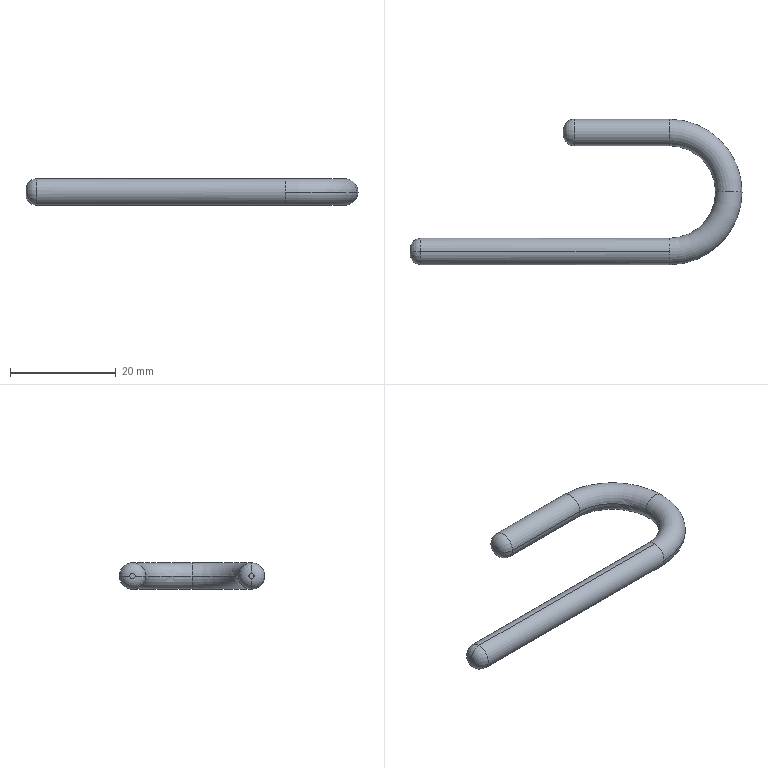Part | STEP file | 10000020444swp000-1 | 1 solid | 14 faces | box 62.75 x 27.5 x 5 mm | volume 2027 mm3 | torus 8 | cylinder 4 | plane 2 | commonest cylinder face diameters 5 x4
STEP:
#1=CARTESIAN_POINT('',(62.75,11.25,0.));
#2=VERTEX_POINT('',#1);
#3=CARTESIAN_POINT('',(57.75,11.25,0.));
#4=VERTEX_POINT('',#3);
#5=CARTESIAN_POINT('',(60.25,11.25,0.));
#6=DIRECTION('',(0.,-1.,0.));
#7=DIRECTION('',(0.,0.,-1.));
#8=AXIS2_PLACEMENT_3D('',#5,#6,#7);
#9=CIRCLE('',#8,2.5);
#10=EDGE_CURVE('',#2,#4,#9,.T.);
#11=ORIENTED_EDGE('',*,*,#10,.F.);
#12=CARTESIAN_POINT('',(49.,25.,0.));
#13=VERTEX_POINT('',#12);
#14=CARTESIAN_POINT('',(49.,11.25,0.));
#15=DIRECTION('',(0.,0.,1.));
#16=DIRECTION('',(1.,0.,0.));
#17=AXIS2_PLACEMENT_3D('',#14,#15,#16);
#18=CIRCLE('',#17,13.75);
#19=EDGE_CURVE('',#2,#13,#18,.T.);
#20=ORIENTED_EDGE('',*,*,#19,.T.);
#21=CARTESIAN_POINT('',(49.,20.,0.));
#22=VERTEX_POINT('',#21);
#23=CARTESIAN_POINT('',(49.,22.5,0.));
#24=DIRECTION('',(-1.,0.,0.));
#25=DIRECTION('',(0.,0.,-1.));
#26=AXIS2_PLACEMENT_3D('',#23,#24,#25);
#27=CIRCLE('',#26,2.5);
#28=EDGE_CURVE('',#22,#13,#27,.T.);
#29=ORIENTED_EDGE('',*,*,#28,.F.);
#30=CARTESIAN_POINT('',(49.,11.25,0.));
#31=DIRECTION('',(0.,0.,1.));
#32=DIRECTION('',(1.,0.,0.));
#33=AXIS2_PLACEMENT_3D('',#30,#31,#32);
#34=CIRCLE('',#33,8.75);
#35=EDGE_CURVE('',#4,#22,#34,.T.);
#36=ORIENTED_EDGE('',*,*,#35,.F.);
#37=EDGE_LOOP('',(#11,#20,#29,#36));
#38=FACE_OUTER_BOUND('',#37,.T.);
#39=CARTESIAN_POINT('',(49.,11.25,0.));
#40=DIRECTION('',(0.,0.,1.));
#41=DIRECTION('',(1.,0.,0.));
#42=AXIS2_PLACEMENT_3D('',#39,#40,#41);
#43=TOROIDAL_SURFACE('',#42,11.25,2.5);
#44=ADVANCED_FACE('',(#38),#43,.T.);
#45=CARTESIAN_POINT('',(49.,0.,2.5));
#46=VERTEX_POINT('',#45);
#47=CARTESIAN_POINT('',(49.,-2.5,0.));
#48=VERTEX_POINT('',#47);
#49=CARTESIAN_POINT('',(49.,0.,0.));
#50=DIRECTION('',(1.,0.,0.));
#51=DIRECTION('',(0.,0.,-1.));
#52=AXIS2_PLACEMENT_3D('',#49,#50,#51);
#53=CIRCLE('',#52,2.5);
#54=EDGE_CURVE('',#46,#48,#53,.T.);
#55=ORIENTED_EDGE('',*,*,#54,.T.);
#56=CARTESIAN_POINT('',(49.,11.25,0.));
#57=DIRECTION('',(0.,0.,1.));
#58=DIRECTION('',(1.,0.,0.));
#59=AXIS2_PLACEMENT_3D('',#56,#57,#58);
#60=CIRCLE('',#59,13.75);
#61=EDGE_CURVE('',#48,#2,#60,.T.);
#62=ORIENTED_EDGE('',*,*,#61,.T.);
#63=ORIENTED_EDGE('',*,*,#10,.T.);
#64=CARTESIAN_POINT('',(49.,2.5,0.));
#65=VERTEX_POINT('',#64);
#66=CARTESIAN_POINT('',(49.,11.25,0.));
#67=DIRECTION('',(0.,0.,1.));
#68=DIRECTION('',(1.,0.,0.));
#69=AXIS2_PLACEMENT_3D('',#66,#67,#68);
#70=CIRCLE('',#69,8.75);
#71=EDGE_CURVE('',#65,#4,#70,.T.);
#72=ORIENTED_EDGE('',*,*,#71,.F.);
#73=CARTESIAN_POINT('',(49.,0.,0.));
#74=DIRECTION('',(1.,0.,0.));
#75=DIRECTION('',(0.,0.,-1.));
#76=AXIS2_PLACEMENT_3D('',#73,#74,#75);
#77=CIRCLE('',#76,2.5);
#78=EDGE_CURVE('',#65,#46,#77,.T.);
#79=ORIENTED_EDGE('',*,*,#78,.T.);
#80=EDGE_LOOP('',(#55,#62,#63,#72,#79));
#81=FACE_OUTER_BOUND('',#80,.T.);
#82=CARTESIAN_POINT('',(49.,11.25,0.));
#83=DIRECTION('',(0.,0.,1.));
#84=DIRECTION('',(1.,0.,0.));
#85=AXIS2_PLACEMENT_3D('',#82,#83,#84);
#86=TOROIDAL_SURFACE('',#85,11.25,2.5);
#87=ADVANCED_FACE('',(#81),#86,.T.);
#88=CARTESIAN_POINT('',(0.,0.,0.5));
#89=VERTEX_POINT('',#88);
#90=CARTESIAN_POINT('',(0.,0.,-0.5));
#91=VERTEX_POINT('',#90);
#92=CARTESIAN_POINT('',(0.,0.,0.));
#93=DIRECTION('',(-1.,0.,0.));
#94=DIRECTION('',(0.,0.,-1.));
#95=AXIS2_PLACEMENT_3D('',#92,#93,#94);
#96=CIRCLE('',#95,0.5);
#97=EDGE_CURVE('',#89,#91,#96,.T.);
#98=ORIENTED_EDGE('',*,*,#97,.F.);
#99=CARTESIAN_POINT('',(2.,0.,2.5));
#100=VERTEX_POINT('',#99);
#101=CARTESIAN_POINT('',(2.,0.,0.5));
#102=DIRECTION('',(0.,1.,0.));
#103=DIRECTION('',(0.,0.,1.));
#104=AXIS2_PLACEMENT_3D('',#101,#102,#103);
#105=CIRCLE('',#104,2.);
#106=EDGE_CURVE('',#89,#100,#105,.T.);
#107=ORIENTED_EDGE('',*,*,#106,.T.);
#108=CARTESIAN_POINT('',(2.,0.,-2.5));
#109=VERTEX_POINT('',#108);
#110=CARTESIAN_POINT('',(2.,0.,0.));
#111=DIRECTION('',(1.,0.,0.));
#112=DIRECTION('',(0.,0.,-1.));
#113=AXIS2_PLACEMENT_3D('',#110,#111,#112);
#114=CIRCLE('',#113,2.5);
#115=EDGE_CURVE('',#109,#100,#114,.T.);
#116=ORIENTED_EDGE('',*,*,#115,.F.);
#117=CARTESIAN_POINT('',(2.,0.,-0.5));
#118=DIRECTION('',(0.,-1.,0.));
#119=DIRECTION('',(0.,0.,-1.));
#120=AXIS2_PLACEMENT_3D('',#117,#118,#119);
#121=CIRCLE('',#120,2.);
#122=EDGE_CURVE('',#91,#109,#121,.T.);
#123=ORIENTED_EDGE('',*,*,#122,.F.);
#124=EDGE_LOOP('',(#98,#107,#116,#123));
#125=FACE_OUTER_BOUND('',#124,.T.);
#126=CARTESIAN_POINT('',(2.,0.,0.));
#127=DIRECTION('',(1.,0.,0.));
#128=DIRECTION('',(0.,0.,-1.));
#129=AXIS2_PLACEMENT_3D('',#126,#127,#128);
#130=TOROIDAL_SURFACE('',#129,0.5,2.);
#131=ADVANCED_FACE('',(#125),#130,.T.);
#132=CARTESIAN_POINT('',(31.,25.,0.));
#133=VERTEX_POINT('',#132);
#134=CARTESIAN_POINT('',(31.,20.,0.));
#135=VERTEX_POINT('',#134);
#136=CARTESIAN_POINT('',(31.,22.5,0.));
#137=DIRECTION('',(1.,0.,0.));
#138=DIRECTION('',(0.,-1.,0.));
#139=AXIS2_PLACEMENT_3D('',#136,#137,#138);
#140=CIRCLE('',#139,2.5);
#141=EDGE_CURVE('',#133,#135,#140,.T.);
#142=ORIENTED_EDGE('',*,*,#141,.F.);
#143=CARTESIAN_POINT('',(29.,23.,0.));
#144=VERTEX_POINT('',#143);
#145=CARTESIAN_POINT('',(31.,23.,0.));
#146=DIRECTION('',(0.,0.,1.));
#147=DIRECTION('',(0.,-1.,0.));
#148=AXIS2_PLACEMENT_3D('',#145,#146,#147);
#149=CIRCLE('',#148,2.);
#150=EDGE_CURVE('',#133,#144,#149,.T.);
#151=ORIENTED_EDGE('',*,*,#150,.T.);
#152=CARTESIAN_POINT('',(29.,22.,0.));
#153=VERTEX_POINT('',#152);
#154=CARTESIAN_POINT('',(29.,22.5,0.));
#155=DIRECTION('',(-1.,0.,0.));
#156=DIRECTION('',(0.,-1.,0.));
#157=AXIS2_PLACEMENT_3D('',#154,#155,#156);
#158=CIRCLE('',#157,0.5);
#159=EDGE_CURVE('',#153,#144,#158,.T.);
#160=ORIENTED_EDGE('',*,*,#159,.F.);
#161=CARTESIAN_POINT('',(31.,22.,0.));
#162=DIRECTION('',(0.,0.,-1.));
#163=DIRECTION('',(-1.,0.,0.));
#164=AXIS2_PLACEMENT_3D('',#161,#162,#163);
#165=CIRCLE('',#164,2.);
#166=EDGE_CURVE('',#135,#153,#165,.T.);
#167=ORIENTED_EDGE('',*,*,#166,.F.);
#168=EDGE_LOOP('',(#142,#151,#160,#167));
#169=FACE_OUTER_BOUND('',#168,.T.);
#170=CARTESIAN_POINT('',(31.,22.5,0.));
#171=DIRECTION('',(-1.,0.,0.));
#172=DIRECTION('',(0.,-1.,0.));
#173=AXIS2_PLACEMENT_3D('',#170,#171,#172);
#174=TOROIDAL_SURFACE('',#173,0.5,2.);
#175=ADVANCED_FACE('',(#169),#174,.T.);
#176=CARTESIAN_POINT('',(49.,0.,-2.5));
#177=VERTEX_POINT('',#176);
#178=CARTESIAN_POINT('',(49.,0.,0.));
#179=DIRECTION('',(1.,0.,0.));
#180=DIRECTION('',(0.,0.,-1.));
#181=AXIS2_PLACEMENT_3D('',#178,#179,#180);
#182=CIRCLE('',#181,2.5);
#183=EDGE_CURVE('',#177,#65,#182,.T.);
#184=ORIENTED_EDGE('',*,*,#183,.F.);
#185=CARTESIAN_POINT('',(49.,0.,-2.5));
#186=DIRECTION('',(-1.,0.,0.));
#187=VECTOR('',#186,1000.);
#188=LINE('',#185,#187);
#189=EDGE_CURVE('',#177,#109,#188,.T.);
#190=ORIENTED_EDGE('',*,*,#189,.T.);
#191=ORIENTED_EDGE('',*,*,#115,.T.);
#192=CARTESIAN_POINT('',(49.,0.,2.5));
#193=DIRECTION('',(-1.,0.,0.));
#194=VECTOR('',#193,1000.);
#195=LINE('',#192,#194);
#196=EDGE_CURVE('',#46,#100,#195,.T.);
#197=ORIENTED_EDGE('',*,*,#196,.F.);
#198=ORIENTED_EDGE('',*,*,#78,.F.);
#199=EDGE_LOOP('',(#184,#190,#191,#197,#198));
#200=FACE_OUTER_BOUND('',#199,.T.);
#201=CARTESIAN_POINT('',(49.,0.,0.));
#202=DIRECTION('',(-1.,0.,0.));
#203=DIRECTION('',(0.,0.,1.));
#204=AXIS2_PLACEMENT_3D('',#201,#202,#203);
#205=CYLINDRICAL_SURFACE('',#204,2.5);
#206=ADVANCED_FACE('',(#200),#205,.T.);
#207=ORIENTED_EDGE('',*,*,#61,.F.);
#208=CARTESIAN_POINT('',(49.,0.,0.));
#209=DIRECTION('',(1.,0.,0.));
#210=DIRECTION('',(0.,0.,-1.));
#211=AXIS2_PLACEMENT_3D('',#208,#209,#210);
#212=CIRCLE('',#211,2.5);
#213=EDGE_CURVE('',#48,#177,#212,.T.);
#214=ORIENTED_EDGE('',*,*,#213,.T.);
#215=ORIENTED_EDGE('',*,*,#183,.T.);
#216=ORIENTED_EDGE('',*,*,#71,.T.);
#217=CARTESIAN_POINT('',(60.25,11.25,0.));
#218=DIRECTION('',(0.,-1.,0.));
#219=DIRECTION('',(0.,0.,-1.));
#220=AXIS2_PLACEMENT_3D('',#217,#218,#219);
#221=CIRCLE('',#220,2.5);
#222=EDGE_CURVE('',#4,#2,#221,.T.);
#223=ORIENTED_EDGE('',*,*,#222,.T.);
#224=EDGE_LOOP('',(#207,#214,#215,#216,#223));
#225=FACE_OUTER_BOUND('',#224,.T.);
#226=CARTESIAN_POINT('',(49.,11.25,0.));
#227=DIRECTION('',(0.,0.,1.));
#228=DIRECTION('',(1.,0.,0.));
#229=AXIS2_PLACEMENT_3D('',#226,#227,#228);
#230=TOROIDAL_SURFACE('',#229,11.25,2.5);
#231=ADVANCED_FACE('',(#225),#230,.T.);
#232=ORIENTED_EDGE('',*,*,#28,.T.);
#233=CARTESIAN_POINT('',(49.,25.,0.));
#234=DIRECTION('',(-1.,0.,0.));
#235=VECTOR('',#234,1000.);
#236=LINE('',#233,#235);
#237=EDGE_CURVE('',#13,#133,#236,.T.);
#238=ORIENTED_EDGE('',*,*,#237,.T.);
#239=ORIENTED_EDGE('',*,*,#141,.T.);
#240=CARTESIAN_POINT('',(49.,20.,0.));
#241=DIRECTION('',(-1.,0.,0.));
#242=VECTOR('',#241,1000.);
#243=LINE('',#240,#242);
#244=EDGE_CURVE('',#22,#135,#243,.T.);
#245=ORIENTED_EDGE('',*,*,#244,.F.);
#246=EDGE_LOOP('',(#232,#238,#239,#245));
#247=FACE_OUTER_BOUND('',#246,.T.);
#248=CARTESIAN_POINT('',(49.,22.5,0.));
#249=DIRECTION('',(-1.,0.,0.));
#250=DIRECTION('',(0.,-1.,0.));
#251=AXIS2_PLACEMENT_3D('',#248,#249,#250);
#252=CYLINDRICAL_SURFACE('',#251,2.5);
#253=ADVANCED_FACE('',(#247),#252,.T.);
#254=ORIENTED_EDGE('',*,*,#237,.F.);
#255=CARTESIAN_POINT('',(49.,22.5,0.));
#256=DIRECTION('',(-1.,0.,0.));
#257=DIRECTION('',(0.,0.,-1.));
#258=AXIS2_PLACEMENT_3D('',#255,#256,#257);
#259=CIRCLE('',#258,2.5);
#260=EDGE_CURVE('',#13,#22,#259,.T.);
#261=ORIENTED_EDGE('',*,*,#260,.T.);
#262=ORIENTED_EDGE('',*,*,#244,.T.);
#263=CARTESIAN_POINT('',(31.,22.5,0.));
#264=DIRECTION('',(1.,0.,0.));
#265=DIRECTION('',(0.,-1.,0.));
#266=AXIS2_PLACEMENT_3D('',#263,#264,#265);
#267=CIRCLE('',#266,2.5);
#268=EDGE_CURVE('',#135,#133,#267,.T.);
#269=ORIENTED_EDGE('',*,*,#268,.T.);
#270=EDGE_LOOP('',(#254,#261,#262,#269));
#271=FACE_OUTER_BOUND('',#270,.T.);
#272=CARTESIAN_POINT('',(49.,22.5,0.));
#273=DIRECTION('',(-1.,0.,0.));
#274=DIRECTION('',(0.,-1.,0.));
#275=AXIS2_PLACEMENT_3D('',#272,#273,#274);
#276=CYLINDRICAL_SURFACE('',#275,2.5);
#277=ADVANCED_FACE('',(#271),#276,.T.);
#278=ORIENTED_EDGE('',*,*,#19,.F.);
#279=ORIENTED_EDGE('',*,*,#222,.F.);
#280=ORIENTED_EDGE('',*,*,#35,.T.);
#281=ORIENTED_EDGE('',*,*,#260,.F.);
#282=EDGE_LOOP('',(#278,#279,#280,#281));
#283=FACE_OUTER_BOUND('',#282,.T.);
#284=CARTESIAN_POINT('',(49.,11.25,0.));
#285=DIRECTION('',(0.,0.,1.));
#286=DIRECTION('',(1.,0.,0.));
#287=AXIS2_PLACEMENT_3D('',#284,#285,#286);
#288=TOROIDAL_SURFACE('',#287,11.25,2.5);
#289=ADVANCED_FACE('',(#283),#288,.T.);
#290=ORIENTED_EDGE('',*,*,#189,.F.);
#291=ORIENTED_EDGE('',*,*,#213,.F.);
#292=ORIENTED_EDGE('',*,*,#54,.F.);
#293=ORIENTED_EDGE('',*,*,#196,.T.);
#294=CARTESIAN_POINT('',(2.,0.,0.));
#295=DIRECTION('',(1.,0.,0.));
#296=DIRECTION('',(0.,0.,-1.));
#297=AXIS2_PLACEMENT_3D('',#294,#295,#296);
#298=CIRCLE('',#297,2.5);
#299=EDGE_CURVE('',#100,#109,#298,.T.);
#300=ORIENTED_EDGE('',*,*,#299,.T.);
#301=EDGE_LOOP('',(#290,#291,#292,#293,#300));
#302=FACE_OUTER_BOUND('',#301,.T.);
#303=CARTESIAN_POINT('',(49.,0.,0.));
#304=DIRECTION('',(-1.,0.,0.));
#305=DIRECTION('',(0.,0.,1.));
#306=AXIS2_PLACEMENT_3D('',#303,#304,#305);
#307=CYLINDRICAL_SURFACE('',#306,2.5);
#308=ADVANCED_FACE('',(#302),#307,.T.);
#309=ORIENTED_EDGE('',*,*,#159,.T.);
#310=CARTESIAN_POINT('',(29.,22.5,0.));
#311=DIRECTION('',(-1.,0.,0.));
#312=DIRECTION('',(0.,-1.,0.));
#313=AXIS2_PLACEMENT_3D('',#310,#311,#312);
#314=CIRCLE('',#313,0.5);
#315=EDGE_CURVE('',#144,#153,#314,.T.);
#316=ORIENTED_EDGE('',*,*,#315,.T.);
#317=EDGE_LOOP('',(#309,#316));
#318=FACE_OUTER_BOUND('',#317,.T.);
#319=CARTESIAN_POINT('',(29.,22.5,0.));
#320=DIRECTION('',(-1.,0.,0.));
#321=DIRECTION('',(0.,0.,-1.));
#322=AXIS2_PLACEMENT_3D('',#319,#320,#321);
#323=PLANE('',#322);
#324=ADVANCED_FACE('',(#318),#323,.T.);
#325=CARTESIAN_POINT('',(0.,0.,0.));
#326=DIRECTION('',(-1.,0.,0.));
#327=DIRECTION('',(0.,0.,-1.));
#328=AXIS2_PLACEMENT_3D('',#325,#326,#327);
#329=CIRCLE('',#328,0.5);
#330=EDGE_CURVE('',#91,#89,#329,.T.);
#331=ORIENTED_EDGE('',*,*,#330,.T.);
#332=ORIENTED_EDGE('',*,*,#97,.T.);
#333=EDGE_LOOP('',(#331,#332));
#334=FACE_OUTER_BOUND('',#333,.T.);
#335=CARTESIAN_POINT('',(0.,0.,0.));
#336=DIRECTION('',(1.,0.,0.));
#337=DIRECTION('',(0.,0.,-1.));
#338=AXIS2_PLACEMENT_3D('',#335,#336,#337);
#339=PLANE('',#338);
#340=ADVANCED_FACE('',(#334),#339,.F.);
#341=ORIENTED_EDGE('',*,*,#150,.F.);
#342=ORIENTED_EDGE('',*,*,#268,.F.);
#343=ORIENTED_EDGE('',*,*,#166,.T.);
#344=ORIENTED_EDGE('',*,*,#315,.F.);
#345=EDGE_LOOP('',(#341,#342,#343,#344));
#346=FACE_OUTER_BOUND('',#345,.T.);
#347=CARTESIAN_POINT('',(31.,22.5,0.));
#348=DIRECTION('',(-1.,0.,0.));
#349=DIRECTION('',(0.,-1.,0.));
#350=AXIS2_PLACEMENT_3D('',#347,#348,#349);
#351=TOROIDAL_SURFACE('',#350,0.5,2.);
#352=ADVANCED_FACE('',(#346),#351,.T.);
#353=ORIENTED_EDGE('',*,*,#106,.F.);
#354=ORIENTED_EDGE('',*,*,#330,.F.);
#355=ORIENTED_EDGE('',*,*,#122,.T.);
#356=ORIENTED_EDGE('',*,*,#299,.F.);
#357=EDGE_LOOP('',(#353,#354,#355,#356));
#358=FACE_OUTER_BOUND('',#357,.T.);
#359=CARTESIAN_POINT('',(2.,0.,0.));
#360=DIRECTION('',(1.,0.,0.));
#361=DIRECTION('',(0.,0.,-1.));
#362=AXIS2_PLACEMENT_3D('',#359,#360,#361);
#363=TOROIDAL_SURFACE('',#362,0.5,2.);
#364=ADVANCED_FACE('',(#358),#363,.T.);
#365=CLOSED_SHELL('',(#44,#87,#131,#175,#206,#231,#253,#277,#289,#308,#324,#340,#352,#364));
#366=MANIFOLD_SOLID_BREP('',#365);
#367=CARTESIAN_POINT('',(0.,0.,0.));
#368=DIRECTION('',(0.,0.,1.));
#369=DIRECTION('',(1.,0.,0.));
#370=AXIS2_PLACEMENT_3D('',#367,#368,#369);
#371=(LENGTH_UNIT()NAMED_UNIT(*)SI_UNIT(.MILLI.,.METRE.));
#372=UNCERTAINTY_MEASURE_WITH_UNIT(LENGTH_MEASURE(0.00001),#371,'','');
#373=(NAMED_UNIT(*)PLANE_ANGLE_UNIT()SI_UNIT($,.RADIAN.));
#374=(NAMED_UNIT(*)SI_UNIT($,.STERADIAN.)SOLID_ANGLE_UNIT());
#375=(GEOMETRIC_REPRESENTATION_CONTEXT(3)GLOBAL_UNCERTAINTY_ASSIGNED_CONTEXT((#372))GLOBAL_UNIT_ASSIGNED_CONTEXT((#371,#373,#374))REPRESENTATION_CONTEXT('',''));
#376=ADVANCED_BREP_SHAPE_REPRESENTATION('',(#366,#370),#375);